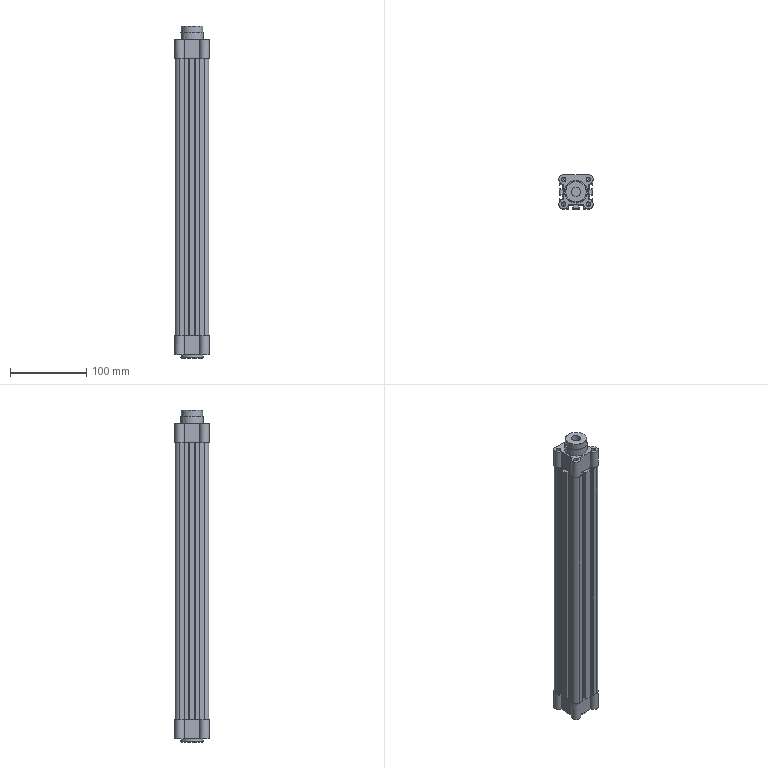Part | STEP file | 163314 DNC-32-320-PPV-A---(FESTO)_CORPO | 1 solid | 184 faces | box 45 x 45 x 436 mm | volume 470774 mm3 | cylinder 83 | plane 81 | cone 20 | commonest cylinder face diameters 0.6 x24 0.8 x24 12.5 x12 4.917 x8 6 x8 8.566 x2